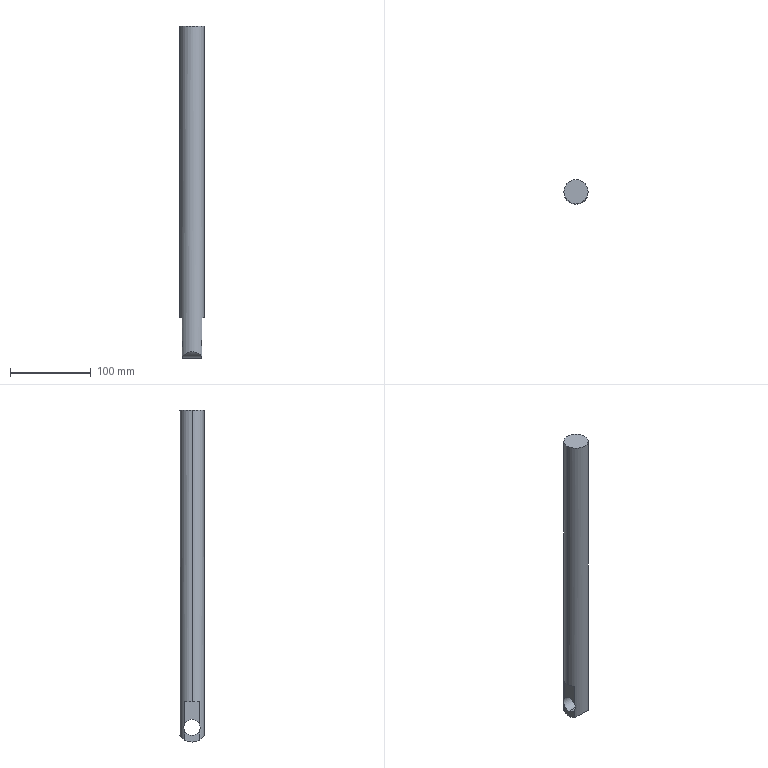Part | STEP file | Hydraulic cylinder B-500 | 1 solid | 13 faces | box 30 x 30 x 411 mm | volume 278111 mm3 | plane 7 | cylinder 6 | commonest cylinder face diameters 20 x2 30 x2 36 x2
STEP:
#1=CARTESIAN_POINT('',(15.,0.,411.));
#2=VERTEX_POINT('',#1);
#3=CARTESIAN_POINT('',(-15.,0.,411.));
#4=VERTEX_POINT('',#3);
#5=CARTESIAN_POINT('',(0.,0.,411.));
#6=DIRECTION('',(0.,0.,1.));
#7=DIRECTION('',(1.,0.,0.));
#8=AXIS2_PLACEMENT_3D('',#5,#6,#7);
#9=CIRCLE('',#8,15.);
#10=EDGE_CURVE('',#2,#4,#9,.T.);
#11=ORIENTED_EDGE('',*,*,#10,.F.);
#12=CARTESIAN_POINT('',(15.,0.,50.));
#13=VERTEX_POINT('',#12);
#14=CARTESIAN_POINT('',(15.,0.,300.));
#15=DIRECTION('',(0.,0.,-1.));
#16=VECTOR('',#15,1000.);
#17=LINE('',#14,#16);
#18=EDGE_CURVE('',#2,#13,#17,.T.);
#19=ORIENTED_EDGE('',*,*,#18,.T.);
#20=CARTESIAN_POINT('',(12.,9.,50.));
#21=VERTEX_POINT('',#20);
#22=CARTESIAN_POINT('',(0.,0.,50.));
#23=DIRECTION('',(0.,0.,1.));
#24=DIRECTION('',(-1.,0.,0.));
#25=AXIS2_PLACEMENT_3D('',#22,#23,#24);
#26=CIRCLE('',#25,15.);
#27=EDGE_CURVE('',#13,#21,#26,.T.);
#28=ORIENTED_EDGE('',*,*,#27,.T.);
#29=CARTESIAN_POINT('',(12.,9.,22.359));
#30=VERTEX_POINT('',#29);
#31=CARTESIAN_POINT('',(12.,9.,300.));
#32=DIRECTION('',(0.,0.,-1.));
#33=VECTOR('',#32,1000.);
#34=LINE('',#31,#33);
#35=EDGE_CURVE('',#21,#30,#34,.T.);
#36=ORIENTED_EDGE('',*,*,#35,.T.);
#37=CARTESIAN_POINT('',(12.,9.,13.641));
#38=VERTEX_POINT('',#37);
#39=CARTESIAN_POINT('',(12.,9.,22.359));
#40=CARTESIAN_POINT('',(11.76,9.32,21.698));
#41=CARTESIAN_POINT('',(11.555,9.568,21.005));
#42=CARTESIAN_POINT('',(11.336,9.824,19.903));
#43=CARTESIAN_POINT('',(11.277,9.89,19.524));
#44=CARTESIAN_POINT('',(11.2,9.978,18.768));
#45=CARTESIAN_POINT('',(11.181,10.,18.389));
#46=CARTESIAN_POINT('',(11.18,10.,17.627));
#47=CARTESIAN_POINT('',(11.199,9.979,17.243));
#48=CARTESIAN_POINT('',(11.277,9.891,16.479));
#49=CARTESIAN_POINT('',(11.334,9.826,16.106));
#50=CARTESIAN_POINT('',(11.551,9.571,15.008));
#51=CARTESIAN_POINT('',(11.76,9.32,14.303));
#52=CARTESIAN_POINT('',(12.,9.,13.641));
#53=B_SPLINE_CURVE_WITH_KNOTS('',3,(#39,#40,#41,#42,#43,#44,#45,#46,#47,#48,#49,#50,#51,#52),.UNSPECIFIED.,.F.,.F.,(4,2,2,2,2,2,4),(0.,0.002292,0.003438,0.004584,0.00573,0.006876,0.009168),.UNSPECIFIED.);
#54=EDGE_CURVE('',#30,#38,#53,.T.);
#55=ORIENTED_EDGE('',*,*,#54,.T.);
#56=CARTESIAN_POINT('',(12.,9.,2.412));
#57=VERTEX_POINT('',#56);
#58=CARTESIAN_POINT('',(12.,9.,300.));
#59=DIRECTION('',(0.,0.,-1.));
#60=VECTOR('',#59,1000.);
#61=LINE('',#58,#60);
#62=EDGE_CURVE('',#38,#57,#61,.T.);
#63=ORIENTED_EDGE('',*,*,#62,.T.);
#64=CARTESIAN_POINT('',(-12.,9.,2.412));
#65=VERTEX_POINT('',#64);
#66=CARTESIAN_POINT('',(12.,9.,2.412));
#67=CARTESIAN_POINT('',(11.307,9.924,2.945));
#68=CARTESIAN_POINT('',(10.538,10.732,3.52));
#69=CARTESIAN_POINT('',(9.271,11.805,4.404));
#70=CARTESIAN_POINT('',(8.829,12.139,4.702));
#71=CARTESIAN_POINT('',(7.904,12.761,5.298));
#72=CARTESIAN_POINT('',(7.42,13.049,5.595));
#73=CARTESIAN_POINT('',(6.422,13.568,6.165));
#74=CARTESIAN_POINT('',(5.906,13.8,6.439));
#75=CARTESIAN_POINT('',(5.1,14.109,6.822));
#76=CARTESIAN_POINT('',(4.826,14.206,6.944));
#77=CARTESIAN_POINT('',(4.265,14.384,7.177));
#78=CARTESIAN_POINT('',(3.978,14.466,7.288));
#79=CARTESIAN_POINT('',(3.102,14.688,7.592));
#80=CARTESIAN_POINT('',(2.504,14.803,7.758));
#81=CARTESIAN_POINT('',(1.58,14.92,7.93));
#82=CARTESIAN_POINT('',(1.267,14.95,7.975));
#83=CARTESIAN_POINT('',(0.6324,14.99,8.035));
#84=CARTESIAN_POINT('',(0.3154,15.,8.05));
#85=CARTESIAN_POINT('',(-0.63,15.,8.05));
#86=CARTESIAN_POINT('',(-1.255,14.96,7.99));
#87=CARTESIAN_POINT('',(-2.184,14.843,7.818));
#88=CARTESIAN_POINT('',(-2.492,14.795,7.747));
#89=CARTESIAN_POINT('',(-3.094,14.681,7.584));
#90=CARTESIAN_POINT('',(-3.388,14.615,7.493));
#91=CARTESIAN_POINT('',(-4.255,14.396,7.192));
#92=CARTESIAN_POINT('',(-4.813,14.219,6.958));
#93=CARTESIAN_POINT('',(-5.625,13.908,6.573));
#94=CARTESIAN_POINT('',(-5.892,13.797,6.439));
#95=CARTESIAN_POINT('',(-6.412,13.564,6.165));
#96=CARTESIAN_POINT('',(-6.666,13.44,6.025));
#97=CARTESIAN_POINT('',(-7.91,12.794,5.315));
#98=CARTESIAN_POINT('',(-8.825,12.181,4.715));
#99=CARTESIAN_POINT('',(-10.102,11.103,3.824));
#100=CARTESIAN_POINT('',(-10.512,10.716,3.528));
#101=CARTESIAN_POINT('',(-11.287,9.895,2.956));
#102=CARTESIAN_POINT('',(-11.654,9.461,2.678));
#103=CARTESIAN_POINT('',(-12.,9.,2.412));
#104=B_SPLINE_CURVE_WITH_KNOTS('',3,(#66,#67,#68,#69,#70,#71,#72,#73,#74,#75,#76,#77,#78,#79,#80,#81,#82,#83,#84,#85,#86,#87,#88,#89,#90,#91,#92,#93,#94,#95,#96,#97,#98,#99,#100,#101,#102,#103),.UNSPECIFIED.,.F.,.F.,(4,2,2,2,2,2,2,2,2,2,2,2,2,2,2,2,2,2,4),(0.,0.003759,0.005639,0.007518,0.009398,0.01034,0.01128,0.01316,0.0141,0.01504,0.01692,0.01786,0.0188,0.02067,0.02161,0.02255,0.02631,0.02819,0.03007),.UNSPECIFIED.);
#105=EDGE_CURVE('',#57,#65,#104,.T.);
#106=ORIENTED_EDGE('',*,*,#105,.T.);
#107=CARTESIAN_POINT('',(-12.,9.,13.641));
#108=VERTEX_POINT('',#107);
#109=CARTESIAN_POINT('',(-12.,9.,300.));
#110=DIRECTION('',(0.,0.,1.));
#111=VECTOR('',#110,1000.);
#112=LINE('',#109,#111);
#113=EDGE_CURVE('',#65,#108,#112,.T.);
#114=ORIENTED_EDGE('',*,*,#113,.T.);
#115=CARTESIAN_POINT('',(-12.,9.,22.359));
#116=VERTEX_POINT('',#115);
#117=CARTESIAN_POINT('',(-12.,9.,13.641));
#118=CARTESIAN_POINT('',(-11.76,9.32,14.302));
#119=CARTESIAN_POINT('',(-11.555,9.568,14.995));
#120=CARTESIAN_POINT('',(-11.336,9.824,16.097));
#121=CARTESIAN_POINT('',(-11.277,9.89,16.476));
#122=CARTESIAN_POINT('',(-11.2,9.978,17.232));
#123=CARTESIAN_POINT('',(-11.181,10.,17.611));
#124=CARTESIAN_POINT('',(-11.18,10.,18.373));
#125=CARTESIAN_POINT('',(-11.199,9.979,18.757));
#126=CARTESIAN_POINT('',(-11.277,9.891,19.521));
#127=CARTESIAN_POINT('',(-11.334,9.826,19.894));
#128=CARTESIAN_POINT('',(-11.551,9.571,20.992));
#129=CARTESIAN_POINT('',(-11.76,9.32,21.697));
#130=CARTESIAN_POINT('',(-12.,9.,22.359));
#131=B_SPLINE_CURVE_WITH_KNOTS('',3,(#117,#118,#119,#120,#121,#122,#123,#124,#125,#126,#127,#128,#129,#130),.UNSPECIFIED.,.F.,.F.,(4,2,2,2,2,2,4),(0.,0.002292,0.003438,0.004584,0.00573,0.006876,0.009168),.UNSPECIFIED.);
#132=EDGE_CURVE('',#108,#116,#131,.T.);
#133=ORIENTED_EDGE('',*,*,#132,.T.);
#134=CARTESIAN_POINT('',(-12.,9.,50.));
#135=VERTEX_POINT('',#134);
#136=CARTESIAN_POINT('',(-12.,9.,300.));
#137=DIRECTION('',(0.,0.,1.));
#138=VECTOR('',#137,1000.);
#139=LINE('',#136,#138);
#140=EDGE_CURVE('',#116,#135,#139,.T.);
#141=ORIENTED_EDGE('',*,*,#140,.T.);
#142=CARTESIAN_POINT('',(-15.,0.,50.));
#143=VERTEX_POINT('',#142);
#144=CARTESIAN_POINT('',(0.,0.,50.));
#145=DIRECTION('',(0.,0.,1.));
#146=DIRECTION('',(-1.,0.,0.));
#147=AXIS2_PLACEMENT_3D('',#144,#145,#146);
#148=CIRCLE('',#147,15.);
#149=EDGE_CURVE('',#135,#143,#148,.T.);
#150=ORIENTED_EDGE('',*,*,#149,.T.);
#151=CARTESIAN_POINT('',(-15.,0.,300.));
#152=DIRECTION('',(0.,0.,-1.));
#153=VECTOR('',#152,1000.);
#154=LINE('',#151,#153);
#155=EDGE_CURVE('',#4,#143,#154,.T.);
#156=ORIENTED_EDGE('',*,*,#155,.F.);
#157=EDGE_LOOP('',(#11,#19,#28,#36,#55,#63,#106,#114,#133,#141,#150,#156));
#158=FACE_OUTER_BOUND('',#157,.T.);
#159=CARTESIAN_POINT('',(0.,0.,300.));
#160=DIRECTION('',(0.,0.,-1.));
#161=DIRECTION('',(-1.,0.,0.));
#162=AXIS2_PLACEMENT_3D('',#159,#160,#161);
#163=CYLINDRICAL_SURFACE('',#162,15.);
#164=ADVANCED_FACE('',(#158),#163,.T.);
#165=CARTESIAN_POINT('',(-12.,0.,28.));
#166=VERTEX_POINT('',#165);
#167=CARTESIAN_POINT('',(-12.,-9.,22.359));
#168=VERTEX_POINT('',#167);
#169=CARTESIAN_POINT('',(-12.,0.,18.));
#170=DIRECTION('',(1.,0.,0.));
#171=DIRECTION('',(0.,0.,-1.));
#172=AXIS2_PLACEMENT_3D('',#169,#170,#171);
#173=CIRCLE('',#172,10.);
#174=EDGE_CURVE('',#166,#168,#173,.T.);
#175=ORIENTED_EDGE('',*,*,#174,.F.);
#176=CARTESIAN_POINT('',(12.,0.,28.));
#177=VERTEX_POINT('',#176);
#178=CARTESIAN_POINT('',(-15.,0.,28.));
#179=DIRECTION('',(1.,0.,0.));
#180=VECTOR('',#179,1000.);
#181=LINE('',#178,#180);
#182=EDGE_CURVE('',#166,#177,#181,.T.);
#183=ORIENTED_EDGE('',*,*,#182,.T.);
#184=CARTESIAN_POINT('',(12.,-9.,22.359));
#185=VERTEX_POINT('',#184);
#186=CARTESIAN_POINT('',(12.,0.,18.));
#187=DIRECTION('',(-1.,0.,0.));
#188=DIRECTION('',(0.,0.,-1.));
#189=AXIS2_PLACEMENT_3D('',#186,#187,#188);
#190=CIRCLE('',#189,10.);
#191=EDGE_CURVE('',#185,#177,#190,.T.);
#192=ORIENTED_EDGE('',*,*,#191,.F.);
#193=CARTESIAN_POINT('',(12.,-9.,13.641));
#194=VERTEX_POINT('',#193);
#195=CARTESIAN_POINT('',(12.,-9.,13.641));
#196=CARTESIAN_POINT('',(11.76,-9.32,14.302));
#197=CARTESIAN_POINT('',(11.555,-9.568,14.995));
#198=CARTESIAN_POINT('',(11.336,-9.824,16.097));
#199=CARTESIAN_POINT('',(11.277,-9.89,16.476));
#200=CARTESIAN_POINT('',(11.2,-9.978,17.232));
#201=CARTESIAN_POINT('',(11.181,-10.,17.611));
#202=CARTESIAN_POINT('',(11.18,-10.,18.373));
#203=CARTESIAN_POINT('',(11.199,-9.979,18.757));
#204=CARTESIAN_POINT('',(11.277,-9.891,19.521));
#205=CARTESIAN_POINT('',(11.334,-9.826,19.894));
#206=CARTESIAN_POINT('',(11.551,-9.571,20.992));
#207=CARTESIAN_POINT('',(11.76,-9.32,21.697));
#208=CARTESIAN_POINT('',(12.,-9.,22.359));
#209=B_SPLINE_CURVE_WITH_KNOTS('',3,(#195,#196,#197,#198,#199,#200,#201,#202,#203,#204,#205,#206,#207,#208),.UNSPECIFIED.,.F.,.F.,(4,2,2,2,2,2,4),(0.,0.002292,0.003438,0.004584,0.00573,0.006876,0.009168),.UNSPECIFIED.);
#210=EDGE_CURVE('',#194,#185,#209,.T.);
#211=ORIENTED_EDGE('',*,*,#210,.F.);
#212=CARTESIAN_POINT('',(12.,0.,8.));
#213=VERTEX_POINT('',#212);
#214=CARTESIAN_POINT('',(12.,0.,18.));
#215=DIRECTION('',(-1.,0.,0.));
#216=DIRECTION('',(0.,0.,-1.));
#217=AXIS2_PLACEMENT_3D('',#214,#215,#216);
#218=CIRCLE('',#217,10.);
#219=EDGE_CURVE('',#213,#194,#218,.T.);
#220=ORIENTED_EDGE('',*,*,#219,.F.);
#221=CARTESIAN_POINT('',(-12.,0.,8.));
#222=VERTEX_POINT('',#221);
#223=CARTESIAN_POINT('',(-15.,0.,8.));
#224=DIRECTION('',(1.,0.,0.));
#225=VECTOR('',#224,1000.);
#226=LINE('',#223,#225);
#227=EDGE_CURVE('',#222,#213,#226,.T.);
#228=ORIENTED_EDGE('',*,*,#227,.F.);
#229=CARTESIAN_POINT('',(-12.,-9.,13.641));
#230=VERTEX_POINT('',#229);
#231=CARTESIAN_POINT('',(-12.,0.,18.));
#232=DIRECTION('',(1.,0.,0.));
#233=DIRECTION('',(0.,0.,-1.));
#234=AXIS2_PLACEMENT_3D('',#231,#232,#233);
#235=CIRCLE('',#234,10.);
#236=EDGE_CURVE('',#230,#222,#235,.T.);
#237=ORIENTED_EDGE('',*,*,#236,.F.);
#238=CARTESIAN_POINT('',(-12.,-9.,22.359));
#239=CARTESIAN_POINT('',(-11.76,-9.32,21.698));
#240=CARTESIAN_POINT('',(-11.555,-9.568,21.005));
#241=CARTESIAN_POINT('',(-11.336,-9.824,19.903));
#242=CARTESIAN_POINT('',(-11.277,-9.89,19.524));
#243=CARTESIAN_POINT('',(-11.2,-9.978,18.768));
#244=CARTESIAN_POINT('',(-11.181,-10.,18.389));
#245=CARTESIAN_POINT('',(-11.18,-10.,17.627));
#246=CARTESIAN_POINT('',(-11.199,-9.979,17.243));
#247=CARTESIAN_POINT('',(-11.277,-9.891,16.479));
#248=CARTESIAN_POINT('',(-11.334,-9.826,16.106));
#249=CARTESIAN_POINT('',(-11.551,-9.571,15.008));
#250=CARTESIAN_POINT('',(-11.76,-9.32,14.303));
#251=CARTESIAN_POINT('',(-12.,-9.,13.641));
#252=B_SPLINE_CURVE_WITH_KNOTS('',3,(#238,#239,#240,#241,#242,#243,#244,#245,#246,#247,#248,#249,#250,#251),.UNSPECIFIED.,.F.,.F.,(4,2,2,2,2,2,4),(0.,0.002292,0.003438,0.004584,0.00573,0.006876,0.009168),.UNSPECIFIED.);
#253=EDGE_CURVE('',#168,#230,#252,.T.);
#254=ORIENTED_EDGE('',*,*,#253,.F.);
#255=EDGE_LOOP('',(#175,#183,#192,#211,#220,#228,#237,#254));
#256=FACE_OUTER_BOUND('',#255,.T.);
#257=CARTESIAN_POINT('',(-15.,0.,18.));
#258=DIRECTION('',(1.,0.,0.));
#259=DIRECTION('',(0.,0.,-1.));
#260=AXIS2_PLACEMENT_3D('',#257,#258,#259);
#261=CYLINDRICAL_SURFACE('',#260,10.);
#262=ADVANCED_FACE('',(#256),#261,.F.);
#263=CARTESIAN_POINT('',(-12.,0.,0.));
#264=VERTEX_POINT('',#263);
#265=CARTESIAN_POINT('',(-12.,-9.,2.412));
#266=VERTEX_POINT('',#265);
#267=CARTESIAN_POINT('',(-12.,0.,18.));
#268=DIRECTION('',(-1.,0.,0.));
#269=DIRECTION('',(0.,0.,-1.));
#270=AXIS2_PLACEMENT_3D('',#267,#268,#269);
#271=CIRCLE('',#270,18.);
#272=EDGE_CURVE('',#264,#266,#271,.T.);
#273=ORIENTED_EDGE('',*,*,#272,.F.);
#274=CARTESIAN_POINT('',(12.,0.,0.));
#275=VERTEX_POINT('',#274);
#276=CARTESIAN_POINT('',(-28.,0.,0.));
#277=DIRECTION('',(1.,0.,0.));
#278=VECTOR('',#277,1000.);
#279=LINE('',#276,#278);
#280=EDGE_CURVE('',#264,#275,#279,.T.);
#281=ORIENTED_EDGE('',*,*,#280,.T.);
#282=CARTESIAN_POINT('',(12.,-9.,2.412));
#283=VERTEX_POINT('',#282);
#284=CARTESIAN_POINT('',(12.,0.,18.));
#285=DIRECTION('',(-1.,0.,0.));
#286=DIRECTION('',(0.,0.,-1.));
#287=AXIS2_PLACEMENT_3D('',#284,#285,#286);
#288=CIRCLE('',#287,18.);
#289=EDGE_CURVE('',#275,#283,#288,.T.);
#290=ORIENTED_EDGE('',*,*,#289,.T.);
#291=CARTESIAN_POINT('',(-12.,-9.,2.412));
#292=CARTESIAN_POINT('',(-11.307,-9.924,2.945));
#293=CARTESIAN_POINT('',(-10.538,-10.732,3.52));
#294=CARTESIAN_POINT('',(-9.271,-11.805,4.404));
#295=CARTESIAN_POINT('',(-8.829,-12.139,4.702));
#296=CARTESIAN_POINT('',(-7.904,-12.761,5.298));
#297=CARTESIAN_POINT('',(-7.42,-13.049,5.595));
#298=CARTESIAN_POINT('',(-6.422,-13.568,6.165));
#299=CARTESIAN_POINT('',(-5.906,-13.8,6.439));
#300=CARTESIAN_POINT('',(-5.1,-14.109,6.822));
#301=CARTESIAN_POINT('',(-4.826,-14.206,6.944));
#302=CARTESIAN_POINT('',(-4.265,-14.384,7.177));
#303=CARTESIAN_POINT('',(-3.978,-14.466,7.288));
#304=CARTESIAN_POINT('',(-3.102,-14.688,7.592));
#305=CARTESIAN_POINT('',(-2.504,-14.803,7.758));
#306=CARTESIAN_POINT('',(-1.58,-14.92,7.93));
#307=CARTESIAN_POINT('',(-1.267,-14.95,7.975));
#308=CARTESIAN_POINT('',(-0.6324,-14.99,8.035));
#309=CARTESIAN_POINT('',(-0.3154,-15.,8.05));
#310=CARTESIAN_POINT('',(0.63,-15.,8.05));
#311=CARTESIAN_POINT('',(1.255,-14.96,7.99));
#312=CARTESIAN_POINT('',(2.184,-14.843,7.818));
#313=CARTESIAN_POINT('',(2.492,-14.795,7.747));
#314=CARTESIAN_POINT('',(3.094,-14.681,7.584));
#315=CARTESIAN_POINT('',(3.388,-14.615,7.493));
#316=CARTESIAN_POINT('',(4.255,-14.396,7.192));
#317=CARTESIAN_POINT('',(4.813,-14.219,6.958));
#318=CARTESIAN_POINT('',(5.625,-13.908,6.573));
#319=CARTESIAN_POINT('',(5.892,-13.797,6.439));
#320=CARTESIAN_POINT('',(6.412,-13.564,6.165));
#321=CARTESIAN_POINT('',(6.666,-13.44,6.025));
#322=CARTESIAN_POINT('',(7.91,-12.794,5.315));
#323=CARTESIAN_POINT('',(8.825,-12.181,4.715));
#324=CARTESIAN_POINT('',(10.102,-11.103,3.824));
#325=CARTESIAN_POINT('',(10.512,-10.716,3.528));
#326=CARTESIAN_POINT('',(11.287,-9.895,2.956));
#327=CARTESIAN_POINT('',(11.654,-9.461,2.678));
#328=CARTESIAN_POINT('',(12.,-9.,2.412));
#329=B_SPLINE_CURVE_WITH_KNOTS('',3,(#291,#292,#293,#294,#295,#296,#297,#298,#299,#300,#301,#302,#303,#304,#305,#306,#307,#308,#309,#310,#311,#312,#313,#314,#315,#316,#317,#318,#319,#320,#321,#322,#323,#324,#325,#326,#327,#328),.UNSPECIFIED.,.F.,.F.,(4,2,2,2,2,2,2,2,2,2,2,2,2,2,2,2,2,2,4),(0.,0.003759,0.005639,0.007518,0.009398,0.01034,0.01128,0.01316,0.0141,0.01504,0.01692,0.01786,0.0188,0.02067,0.02161,0.02255,0.02631,0.02819,0.03007),.UNSPECIFIED.);
#330=EDGE_CURVE('',#266,#283,#329,.T.);
#331=ORIENTED_EDGE('',*,*,#330,.F.);
#332=EDGE_LOOP('',(#273,#281,#290,#331));
#333=FACE_OUTER_BOUND('',#332,.T.);
#334=CARTESIAN_POINT('',(-28.,0.,18.));
#335=DIRECTION('',(1.,0.,0.));
#336=DIRECTION('',(0.,0.,-1.));
#337=AXIS2_PLACEMENT_3D('',#334,#335,#336);
#338=CYLINDRICAL_SURFACE('',#337,18.);
#339=ADVANCED_FACE('',(#333),#338,.T.);
#340=ORIENTED_EDGE('',*,*,#18,.F.);
#341=CARTESIAN_POINT('',(0.,0.,411.));
#342=DIRECTION('',(0.,0.,1.));
#343=DIRECTION('',(1.,0.,0.));
#344=AXIS2_PLACEMENT_3D('',#341,#342,#343);
#345=CIRCLE('',#344,15.);
#346=EDGE_CURVE('',#4,#2,#345,.T.);
#347=ORIENTED_EDGE('',*,*,#346,.F.);
#348=ORIENTED_EDGE('',*,*,#155,.T.);
#349=CARTESIAN_POINT('',(-12.,-9.,50.));
#350=VERTEX_POINT('',#349);
#351=CARTESIAN_POINT('',(0.,0.,50.));
#352=DIRECTION('',(0.,0.,1.));
#353=DIRECTION('',(-1.,0.,0.));
#354=AXIS2_PLACEMENT_3D('',#351,#352,#353);
#355=CIRCLE('',#354,15.);
#356=EDGE_CURVE('',#143,#350,#355,.T.);
#357=ORIENTED_EDGE('',*,*,#356,.T.);
#358=CARTESIAN_POINT('',(-12.,-9.,300.));
#359=DIRECTION('',(0.,0.,-1.));
#360=VECTOR('',#359,1000.);
#361=LINE('',#358,#360);
#362=EDGE_CURVE('',#350,#168,#361,.T.);
#363=ORIENTED_EDGE('',*,*,#362,.T.);
#364=ORIENTED_EDGE('',*,*,#253,.T.);
#365=CARTESIAN_POINT('',(-12.,-9.,300.));
#366=DIRECTION('',(0.,0.,-1.));
#367=VECTOR('',#366,1000.);
#368=LINE('',#365,#367);
#369=EDGE_CURVE('',#230,#266,#368,.T.);
#370=ORIENTED_EDGE('',*,*,#369,.T.);
#371=ORIENTED_EDGE('',*,*,#330,.T.);
#372=CARTESIAN_POINT('',(12.,-9.,300.));
#373=DIRECTION('',(0.,0.,1.));
#374=VECTOR('',#373,1000.);
#375=LINE('',#372,#374);
#376=EDGE_CURVE('',#283,#194,#375,.T.);
#377=ORIENTED_EDGE('',*,*,#376,.T.);
#378=ORIENTED_EDGE('',*,*,#210,.T.);
#379=CARTESIAN_POINT('',(12.,-9.,50.));
#380=VERTEX_POINT('',#379);
#381=CARTESIAN_POINT('',(12.,-9.,300.));
#382=DIRECTION('',(0.,0.,1.));
#383=VECTOR('',#382,1000.);
#384=LINE('',#381,#383);
#385=EDGE_CURVE('',#185,#380,#384,.T.);
#386=ORIENTED_EDGE('',*,*,#385,.T.);
#387=CARTESIAN_POINT('',(0.,0.,50.));
#388=DIRECTION('',(0.,0.,1.));
#389=DIRECTION('',(-1.,0.,0.));
#390=AXIS2_PLACEMENT_3D('',#387,#388,#389);
#391=CIRCLE('',#390,15.);
#392=EDGE_CURVE('',#380,#13,#391,.T.);
#393=ORIENTED_EDGE('',*,*,#392,.T.);
#394=EDGE_LOOP('',(#340,#347,#348,#357,#363,#364,#370,#371,#377,#378,#386,#393));
#395=FACE_OUTER_BOUND('',#394,.T.);
#396=CARTESIAN_POINT('',(0.,0.,300.));
#397=DIRECTION('',(0.,0.,-1.));
#398=DIRECTION('',(-1.,0.,0.));
#399=AXIS2_PLACEMENT_3D('',#396,#397,#398);
#400=CYLINDRICAL_SURFACE('',#399,15.);
#401=ADVANCED_FACE('',(#395),#400,.T.);
#402=ORIENTED_EDGE('',*,*,#149,.F.);
#403=CARTESIAN_POINT('',(-12.,0.,50.));
#404=DIRECTION('',(0.,-1.,0.));
#405=VECTOR('',#404,1000.);
#406=LINE('',#403,#405);
#407=EDGE_CURVE('',#135,#350,#406,.T.);
#408=ORIENTED_EDGE('',*,*,#407,.T.);
#409=ORIENTED_EDGE('',*,*,#356,.F.);
#410=EDGE_LOOP('',(#402,#408,#409));
#411=FACE_OUTER_BOUND('',#410,.T.);
#412=CARTESIAN_POINT('',(0.,0.,50.));
#413=DIRECTION('',(0.,0.,-1.));
#414=DIRECTION('',(-1.,0.,0.));
#415=AXIS2_PLACEMENT_3D('',#412,#413,#414);
#416=PLANE('',#415);
#417=ADVANCED_FACE('',(#411),#416,.T.);
#418=ORIENTED_EDGE('',*,*,#140,.F.);
#419=CARTESIAN_POINT('',(-12.,0.,18.));
#420=DIRECTION('',(1.,0.,0.));
#421=DIRECTION('',(0.,0.,-1.));
#422=AXIS2_PLACEMENT_3D('',#419,#420,#421);
#423=CIRCLE('',#422,10.);
#424=EDGE_CURVE('',#116,#166,#423,.T.);
#425=ORIENTED_EDGE('',*,*,#424,.T.);
#426=ORIENTED_EDGE('',*,*,#174,.T.);
#427=ORIENTED_EDGE('',*,*,#362,.F.);
#428=ORIENTED_EDGE('',*,*,#407,.F.);
#429=EDGE_LOOP('',(#418,#425,#426,#427,#428));
#430=FACE_OUTER_BOUND('',#429,.T.);
#431=CARTESIAN_POINT('',(-12.,15.,50.));
#432=DIRECTION('',(-1.,0.,0.));
#433=DIRECTION('',(0.,0.,1.));
#434=AXIS2_PLACEMENT_3D('',#431,#432,#433);
#435=PLANE('',#434);
#436=ADVANCED_FACE('',(#430),#435,.T.);
#437=ORIENTED_EDGE('',*,*,#182,.F.);
#438=ORIENTED_EDGE('',*,*,#424,.F.);
#439=ORIENTED_EDGE('',*,*,#132,.F.);
#440=CARTESIAN_POINT('',(-12.,0.,18.));
#441=DIRECTION('',(1.,0.,0.));
#442=DIRECTION('',(0.,0.,-1.));
#443=AXIS2_PLACEMENT_3D('',#440,#441,#442);
#444=CIRCLE('',#443,10.);
#445=EDGE_CURVE('',#222,#108,#444,.T.);
#446=ORIENTED_EDGE('',*,*,#445,.F.);
#447=ORIENTED_EDGE('',*,*,#227,.T.);
#448=CARTESIAN_POINT('',(12.,0.,18.));
#449=DIRECTION('',(-1.,0.,0.));
#450=DIRECTION('',(0.,0.,-1.));
#451=AXIS2_PLACEMENT_3D('',#448,#449,#450);
#452=CIRCLE('',#451,10.);
#453=EDGE_CURVE('',#38,#213,#452,.T.);
#454=ORIENTED_EDGE('',*,*,#453,.F.);
#455=ORIENTED_EDGE('',*,*,#54,.F.);
#456=CARTESIAN_POINT('',(12.,0.,18.));
#457=DIRECTION('',(-1.,0.,0.));
#458=DIRECTION('',(0.,0.,-1.));
#459=AXIS2_PLACEMENT_3D('',#456,#457,#458);
#460=CIRCLE('',#459,10.);
#461=EDGE_CURVE('',#177,#30,#460,.T.);
#462=ORIENTED_EDGE('',*,*,#461,.F.);
#463=EDGE_LOOP('',(#437,#438,#439,#446,#447,#454,#455,#462));
#464=FACE_OUTER_BOUND('',#463,.T.);
#465=CARTESIAN_POINT('',(-15.,0.,18.));
#466=DIRECTION('',(1.,0.,0.));
#467=DIRECTION('',(0.,0.,-1.));
#468=AXIS2_PLACEMENT_3D('',#465,#466,#467);
#469=CYLINDRICAL_SURFACE('',#468,10.);
#470=ADVANCED_FACE('',(#464),#469,.F.);
#471=ORIENTED_EDGE('',*,*,#113,.F.);
#472=CARTESIAN_POINT('',(-12.,0.,18.));
#473=DIRECTION('',(-1.,0.,0.));
#474=DIRECTION('',(0.,0.,-1.));
#475=AXIS2_PLACEMENT_3D('',#472,#473,#474);
#476=CIRCLE('',#475,18.);
#477=EDGE_CURVE('',#65,#264,#476,.T.);
#478=ORIENTED_EDGE('',*,*,#477,.T.);
#479=ORIENTED_EDGE('',*,*,#272,.T.);
#480=ORIENTED_EDGE('',*,*,#369,.F.);
#481=ORIENTED_EDGE('',*,*,#236,.T.);
#482=ORIENTED_EDGE('',*,*,#445,.T.);
#483=EDGE_LOOP('',(#471,#478,#479,#480,#481,#482));
#484=FACE_OUTER_BOUND('',#483,.T.);
#485=CARTESIAN_POINT('',(-12.,15.,50.));
#486=DIRECTION('',(-1.,0.,0.));
#487=DIRECTION('',(0.,0.,1.));
#488=AXIS2_PLACEMENT_3D('',#485,#486,#487);
#489=PLANE('',#488);
#490=ADVANCED_FACE('',(#484),#489,.T.);
#491=ORIENTED_EDGE('',*,*,#280,.F.);
#492=ORIENTED_EDGE('',*,*,#477,.F.);
#493=ORIENTED_EDGE('',*,*,#105,.F.);
#494=CARTESIAN_POINT('',(12.,0.,18.));
#495=DIRECTION('',(-1.,0.,0.));
#496=DIRECTION('',(0.,0.,-1.));
#497=AXIS2_PLACEMENT_3D('',#494,#495,#496);
#498=CIRCLE('',#497,18.);
#499=EDGE_CURVE('',#57,#275,#498,.T.);
#500=ORIENTED_EDGE('',*,*,#499,.T.);
#501=EDGE_LOOP('',(#491,#492,#493,#500));
#502=FACE_OUTER_BOUND('',#501,.T.);
#503=CARTESIAN_POINT('',(-28.,0.,18.));
#504=DIRECTION('',(1.,0.,0.));
#505=DIRECTION('',(0.,0.,-1.));
#506=AXIS2_PLACEMENT_3D('',#503,#504,#505);
#507=CYLINDRICAL_SURFACE('',#506,18.);
#508=ADVANCED_FACE('',(#502),#507,.T.);
#509=ORIENTED_EDGE('',*,*,#453,.T.);
#510=ORIENTED_EDGE('',*,*,#219,.T.);
#511=ORIENTED_EDGE('',*,*,#376,.F.);
#512=ORIENTED_EDGE('',*,*,#289,.F.);
#513=ORIENTED_EDGE('',*,*,#499,.F.);
#514=ORIENTED_EDGE('',*,*,#62,.F.);
#515=EDGE_LOOP('',(#509,#510,#511,#512,#513,#514));
#516=FACE_OUTER_BOUND('',#515,.T.);
#517=CARTESIAN_POINT('',(12.,15.,50.));
#518=DIRECTION('',(1.,0.,0.));
#519=DIRECTION('',(0.,0.,-1.));
#520=AXIS2_PLACEMENT_3D('',#517,#518,#519);
#521=PLANE('',#520);
#522=ADVANCED_FACE('',(#516),#521,.T.);
#523=ORIENTED_EDGE('',*,*,#385,.F.);
#524=ORIENTED_EDGE('',*,*,#191,.T.);
#525=ORIENTED_EDGE('',*,*,#461,.T.);
#526=ORIENTED_EDGE('',*,*,#35,.F.);
#527=CARTESIAN_POINT('',(12.,15.,50.));
#528=DIRECTION('',(0.,-1.,0.));
#529=VECTOR('',#528,1000.);
#530=LINE('',#527,#529);
#531=EDGE_CURVE('',#21,#380,#530,.T.);
#532=ORIENTED_EDGE('',*,*,#531,.T.);
#533=EDGE_LOOP('',(#523,#524,#525,#526,#532));
#534=FACE_OUTER_BOUND('',#533,.T.);
#535=CARTESIAN_POINT('',(12.,15.,50.));
#536=DIRECTION('',(1.,0.,0.));
#537=DIRECTION('',(0.,0.,-1.));
#538=AXIS2_PLACEMENT_3D('',#535,#536,#537);
#539=PLANE('',#538);
#540=ADVANCED_FACE('',(#534),#539,.T.);
#541=ORIENTED_EDGE('',*,*,#392,.F.);
#542=ORIENTED_EDGE('',*,*,#531,.F.);
#543=ORIENTED_EDGE('',*,*,#27,.F.);
#544=EDGE_LOOP('',(#541,#542,#543));
#545=FACE_OUTER_BOUND('',#544,.T.);
#546=CARTESIAN_POINT('',(0.,0.,50.));
#547=DIRECTION('',(0.,0.,-1.));
#548=DIRECTION('',(-1.,0.,0.));
#549=AXIS2_PLACEMENT_3D('',#546,#547,#548);
#550=PLANE('',#549);
#551=ADVANCED_FACE('',(#545),#550,.T.);
#552=ORIENTED_EDGE('',*,*,#346,.T.);
#553=ORIENTED_EDGE('',*,*,#10,.T.);
#554=EDGE_LOOP('',(#552,#553));
#555=FACE_OUTER_BOUND('',#554,.T.);
#556=CARTESIAN_POINT('',(0.,0.,411.));
#557=DIRECTION('',(0.,0.,1.));
#558=DIRECTION('',(1.,0.,0.));
#559=AXIS2_PLACEMENT_3D('',#556,#557,#558);
#560=PLANE('',#559);
#561=ADVANCED_FACE('',(#555),#560,.T.);
#562=CLOSED_SHELL('',(#164,#262,#339,#401,#417,#436,#470,#490,#508,#522,#540,#551,#561));
#563=MANIFOLD_SOLID_BREP('',#562);
#564=CARTESIAN_POINT('',(0.,0.,0.));
#565=DIRECTION('',(0.,0.,1.));
#566=DIRECTION('',(1.,0.,0.));
#567=AXIS2_PLACEMENT_3D('',#564,#565,#566);
#568=(LENGTH_UNIT()NAMED_UNIT(*)SI_UNIT(.MILLI.,.METRE.));
#569=UNCERTAINTY_MEASURE_WITH_UNIT(LENGTH_MEASURE(0.00001),#568,'','');
#570=(NAMED_UNIT(*)PLANE_ANGLE_UNIT()SI_UNIT($,.RADIAN.));
#571=(NAMED_UNIT(*)SI_UNIT($,.STERADIAN.)SOLID_ANGLE_UNIT());
#572=(GEOMETRIC_REPRESENTATION_CONTEXT(3)GLOBAL_UNCERTAINTY_ASSIGNED_CONTEXT((#569))GLOBAL_UNIT_ASSIGNED_CONTEXT((#568,#570,#571))REPRESENTATION_CONTEXT('',''));
#573=ADVANCED_BREP_SHAPE_REPRESENTATION('',(#563,#567),#572);